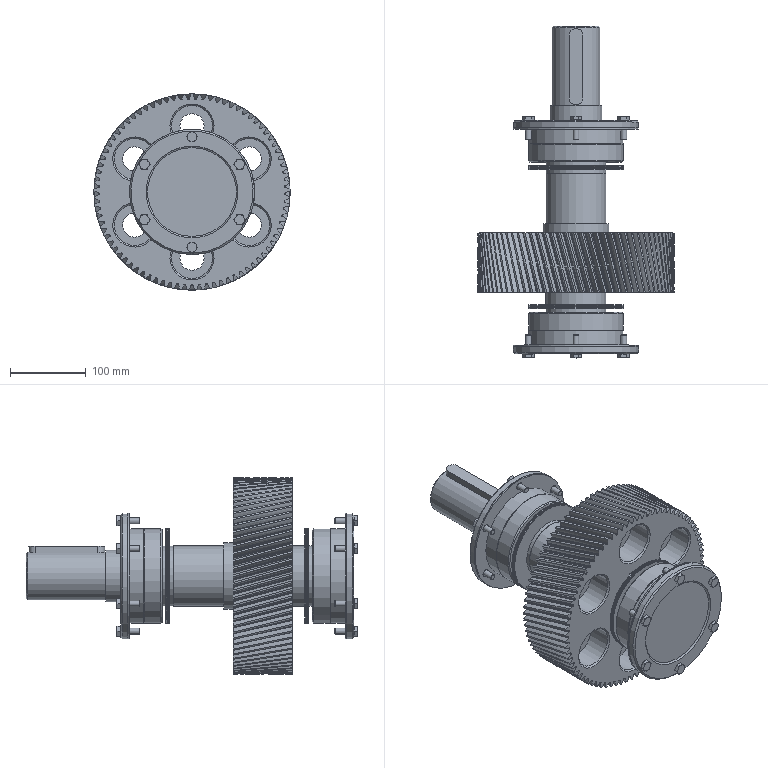Part | NX | 49 solids | 1014 faces | box 258.17 x 436.9 x 258.17 mm | volume 5108197 mm3 | spline 405 | cylinder 192 | plane 189 | cone 186 | sphere 22 | torus 20 | commonest cylinder face diameters 244.67 x81 9 x24 7.76 x12 11.63 x12 54 x12 32 x6